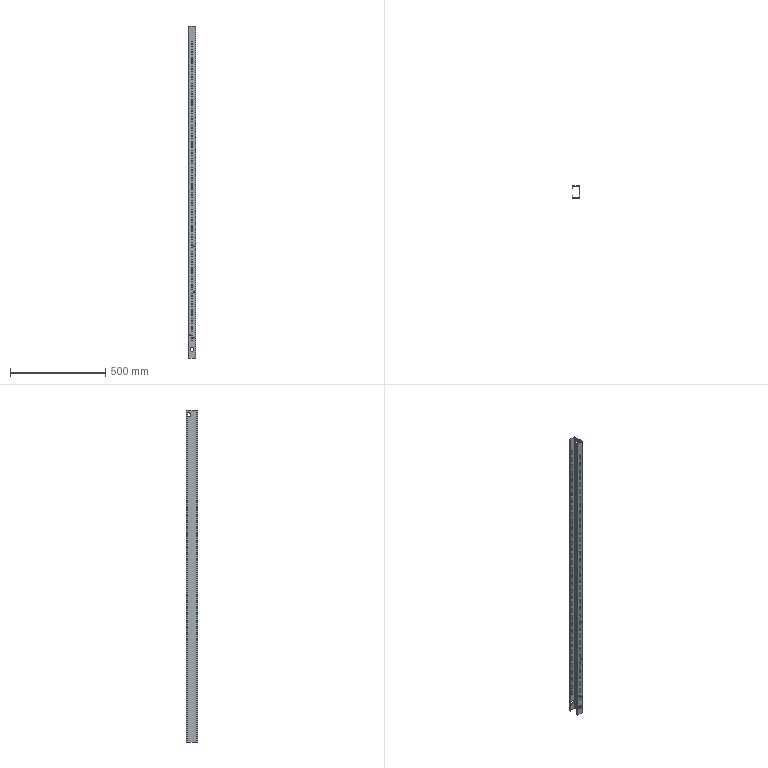Part | STEP file | SOLID | 1 solid | 622 faces | box 37 x 60 x 1739 mm | volume 359493 mm3 | cylinder 312 | plane 310 | commonest cylinder face diameters 3 x144 6.5 x144 3.3 x6 20 x6 0.4 x4 3.4 x4